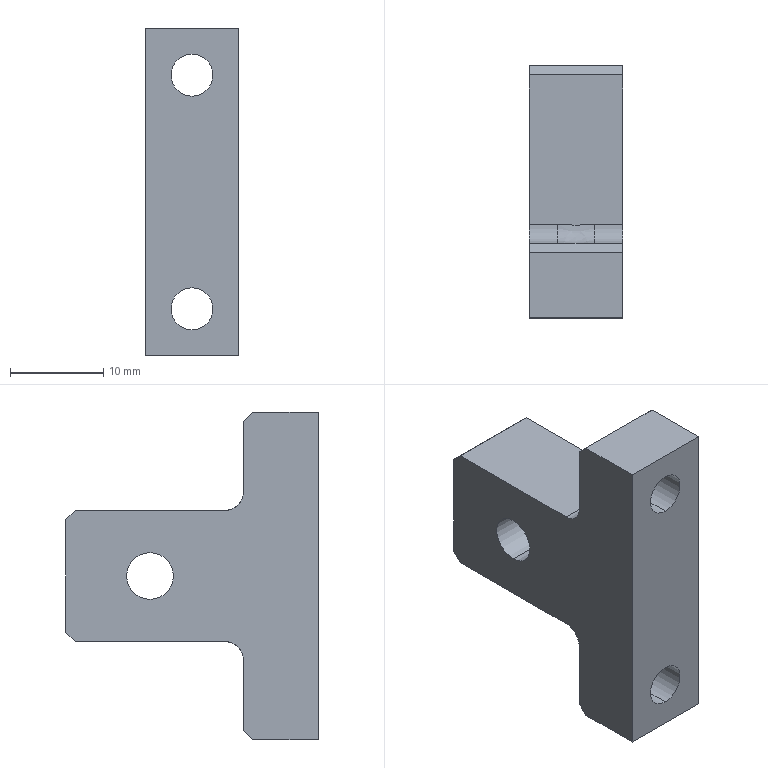Part | SolidWorks | features HoleWzd 2, Chamfer 1, Extrusion 1, Fillet 1 | 1 solid | 34 faces | box 10 x 27 x 35 mm | volume 4690 mm3 | plane 18 | cylinder 14 | spline 2 | commonest cylinder face diameters 4 x4 4.5 x4 8 x4 5 x2
STEP:
#1=CARTESIAN_POINT('',(-5.,18.,2.5));
#2=VERTEX_POINT('',#1);
#3=CARTESIAN_POINT('',(-5.,18.,-2.5));
#4=VERTEX_POINT('',#3);
#5=CARTESIAN_POINT('',(-5.,18.,0.));
#6=DIRECTION('',(1.,0.,0.));
#7=DIRECTION('',(0.,0.,-1.));
#8=AXIS2_PLACEMENT_3D('',#5,#6,#7);
#9=CIRCLE('',#8,2.5);
#10=EDGE_CURVE('',#2,#4,#9,.T.);
#11=ORIENTED_EDGE('',*,*,#10,.F.);
#12=CARTESIAN_POINT('',(5.,18.,2.5));
#13=VERTEX_POINT('',#12);
#14=CARTESIAN_POINT('',(5.,18.,2.5));
#15=DIRECTION('',(1.,0.,0.));
#16=VECTOR('',#15,1000.);
#17=LINE('',#14,#16);
#18=EDGE_CURVE('',#2,#13,#17,.T.);
#19=ORIENTED_EDGE('',*,*,#18,.T.);
#20=CARTESIAN_POINT('',(5.,18.,-2.5));
#21=VERTEX_POINT('',#20);
#22=CARTESIAN_POINT('',(5.,18.,0.));
#23=DIRECTION('',(1.,0.,0.));
#24=DIRECTION('',(0.,0.,-1.));
#25=AXIS2_PLACEMENT_3D('',#22,#23,#24);
#26=CIRCLE('',#25,2.5);
#27=EDGE_CURVE('',#13,#21,#26,.T.);
#28=ORIENTED_EDGE('',*,*,#27,.T.);
#29=CARTESIAN_POINT('',(5.,18.,-2.5));
#30=DIRECTION('',(1.,0.,0.));
#31=VECTOR('',#30,1000.);
#32=LINE('',#29,#31);
#33=EDGE_CURVE('',#4,#21,#32,.T.);
#34=ORIENTED_EDGE('',*,*,#33,.F.);
#35=EDGE_LOOP('',(#11,#19,#28,#34));
#36=FACE_OUTER_BOUND('',#35,.T.);
#37=CARTESIAN_POINT('',(5.,18.,0.));
#38=DIRECTION('',(1.,0.,0.));
#39=DIRECTION('',(0.,0.,-1.));
#40=AXIS2_PLACEMENT_3D('',#37,#38,#39);
#41=CYLINDRICAL_SURFACE('',#40,2.5);
#42=ADVANCED_FACE('',(#36),#41,.F.);
#43=CARTESIAN_POINT('',(0.,3.4,-16.5));
#44=VERTEX_POINT('',#43);
#45=CARTESIAN_POINT('',(0.,3.4,-8.5));
#46=VERTEX_POINT('',#45);
#47=CARTESIAN_POINT('',(0.,3.4,-12.5));
#48=DIRECTION('',(0.,1.,0.));
#49=DIRECTION('',(0.,0.,1.));
#50=AXIS2_PLACEMENT_3D('',#47,#48,#49);
#51=CIRCLE('',#50,4.);
#52=EDGE_CURVE('',#44,#46,#51,.T.);
#53=ORIENTED_EDGE('',*,*,#52,.F.);
#54=CARTESIAN_POINT('',(0.,8.,-16.5));
#55=VERTEX_POINT('',#54);
#56=CARTESIAN_POINT('',(0.,8.,-16.5));
#57=DIRECTION('',(0.,1.,0.));
#58=VECTOR('',#57,1000.);
#59=LINE('',#56,#58);
#60=EDGE_CURVE('',#44,#55,#59,.T.);
#61=ORIENTED_EDGE('',*,*,#60,.T.);
#62=CARTESIAN_POINT('',(-1.936,8.,-9.));
#63=VERTEX_POINT('',#62);
#64=CARTESIAN_POINT('',(0.,8.,-12.5));
#65=DIRECTION('',(0.,1.,0.));
#66=DIRECTION('',(0.,0.,1.));
#67=AXIS2_PLACEMENT_3D('',#64,#65,#66);
#68=CIRCLE('',#67,4.);
#69=EDGE_CURVE('',#55,#63,#68,.T.);
#70=ORIENTED_EDGE('',*,*,#69,.T.);
#71=CARTESIAN_POINT('',(0.,8.,-8.5));
#72=VERTEX_POINT('',#71);
#73=CARTESIAN_POINT('',(0.,8.,-12.5));
#74=DIRECTION('',(0.,1.,0.));
#75=DIRECTION('',(0.,0.,1.));
#76=AXIS2_PLACEMENT_3D('',#73,#74,#75);
#77=CIRCLE('',#76,4.);
#78=EDGE_CURVE('',#63,#72,#77,.T.);
#79=ORIENTED_EDGE('',*,*,#78,.T.);
#80=CARTESIAN_POINT('',(0.,8.,-8.5));
#81=DIRECTION('',(0.,1.,0.));
#82=VECTOR('',#81,1000.);
#83=LINE('',#80,#82);
#84=EDGE_CURVE('',#46,#72,#83,.T.);
#85=ORIENTED_EDGE('',*,*,#84,.F.);
#86=EDGE_LOOP('',(#53,#61,#70,#79,#85));
#87=FACE_OUTER_BOUND('',#86,.T.);
#88=CARTESIAN_POINT('',(0.,8.,-12.5));
#89=DIRECTION('',(0.,1.,0.));
#90=DIRECTION('',(0.,0.,1.));
#91=AXIS2_PLACEMENT_3D('',#88,#89,#90);
#92=CYLINDRICAL_SURFACE('',#91,4.);
#93=ADVANCED_FACE('',(#87),#92,.F.);
#94=CARTESIAN_POINT('',(0.,0.,-14.75));
#95=VERTEX_POINT('',#94);
#96=CARTESIAN_POINT('',(0.,0.,-10.25));
#97=VERTEX_POINT('',#96);
#98=CARTESIAN_POINT('',(0.,0.,-12.5));
#99=DIRECTION('',(0.,1.,0.));
#100=DIRECTION('',(0.,0.,1.));
#101=AXIS2_PLACEMENT_3D('',#98,#99,#100);
#102=CIRCLE('',#101,2.25);
#103=EDGE_CURVE('',#95,#97,#102,.T.);
#104=ORIENTED_EDGE('',*,*,#103,.F.);
#105=CARTESIAN_POINT('',(0.,3.4,-14.75));
#106=VERTEX_POINT('',#105);
#107=CARTESIAN_POINT('',(0.,8.,-14.75));
#108=DIRECTION('',(0.,1.,0.));
#109=VECTOR('',#108,1000.);
#110=LINE('',#107,#109);
#111=EDGE_CURVE('',#95,#106,#110,.T.);
#112=ORIENTED_EDGE('',*,*,#111,.T.);
#113=CARTESIAN_POINT('',(0.,3.4,-10.25));
#114=VERTEX_POINT('',#113);
#115=CARTESIAN_POINT('',(0.,3.4,-12.5));
#116=DIRECTION('',(0.,1.,0.));
#117=DIRECTION('',(0.,0.,1.));
#118=AXIS2_PLACEMENT_3D('',#115,#116,#117);
#119=CIRCLE('',#118,2.25);
#120=EDGE_CURVE('',#106,#114,#119,.T.);
#121=ORIENTED_EDGE('',*,*,#120,.T.);
#122=CARTESIAN_POINT('',(0.,8.,-10.25));
#123=DIRECTION('',(0.,1.,0.));
#124=VECTOR('',#123,1000.);
#125=LINE('',#122,#124);
#126=EDGE_CURVE('',#97,#114,#125,.T.);
#127=ORIENTED_EDGE('',*,*,#126,.F.);
#128=EDGE_LOOP('',(#104,#112,#121,#127));
#129=FACE_OUTER_BOUND('',#128,.T.);
#130=CARTESIAN_POINT('',(0.,8.,-12.5));
#131=DIRECTION('',(0.,1.,0.));
#132=DIRECTION('',(0.,0.,1.));
#133=AXIS2_PLACEMENT_3D('',#130,#131,#132);
#134=CYLINDRICAL_SURFACE('',#133,2.25);
#135=ADVANCED_FACE('',(#129),#134,.F.);
#136=CARTESIAN_POINT('',(0.,3.4,8.5));
#137=VERTEX_POINT('',#136);
#138=CARTESIAN_POINT('',(0.,3.4,16.5));
#139=VERTEX_POINT('',#138);
#140=CARTESIAN_POINT('',(0.,3.4,12.5));
#141=DIRECTION('',(0.,1.,0.));
#142=DIRECTION('',(0.,0.,1.));
#143=AXIS2_PLACEMENT_3D('',#140,#141,#142);
#144=CIRCLE('',#143,4.);
#145=EDGE_CURVE('',#137,#139,#144,.T.);
#146=ORIENTED_EDGE('',*,*,#145,.F.);
#147=CARTESIAN_POINT('',(0.,8.,8.5));
#148=VERTEX_POINT('',#147);
#149=CARTESIAN_POINT('',(0.,8.,8.5));
#150=DIRECTION('',(0.,1.,0.));
#151=VECTOR('',#150,1000.);
#152=LINE('',#149,#151);
#153=EDGE_CURVE('',#137,#148,#152,.T.);
#154=ORIENTED_EDGE('',*,*,#153,.T.);
#155=CARTESIAN_POINT('',(-1.936,8.,9.));
#156=VERTEX_POINT('',#155);
#157=CARTESIAN_POINT('',(0.,8.,12.5));
#158=DIRECTION('',(0.,1.,0.));
#159=DIRECTION('',(0.,0.,1.));
#160=AXIS2_PLACEMENT_3D('',#157,#158,#159);
#161=CIRCLE('',#160,4.);
#162=EDGE_CURVE('',#148,#156,#161,.T.);
#163=ORIENTED_EDGE('',*,*,#162,.T.);
#164=CARTESIAN_POINT('',(0.,8.,16.5));
#165=VERTEX_POINT('',#164);
#166=CARTESIAN_POINT('',(0.,8.,12.5));
#167=DIRECTION('',(0.,1.,0.));
#168=DIRECTION('',(0.,0.,1.));
#169=AXIS2_PLACEMENT_3D('',#166,#167,#168);
#170=CIRCLE('',#169,4.);
#171=EDGE_CURVE('',#156,#165,#170,.T.);
#172=ORIENTED_EDGE('',*,*,#171,.T.);
#173=CARTESIAN_POINT('',(0.,8.,16.5));
#174=DIRECTION('',(0.,1.,0.));
#175=VECTOR('',#174,1000.);
#176=LINE('',#173,#175);
#177=EDGE_CURVE('',#139,#165,#176,.T.);
#178=ORIENTED_EDGE('',*,*,#177,.F.);
#179=EDGE_LOOP('',(#146,#154,#163,#172,#178));
#180=FACE_OUTER_BOUND('',#179,.T.);
#181=CARTESIAN_POINT('',(0.,8.,12.5));
#182=DIRECTION('',(0.,1.,0.));
#183=DIRECTION('',(0.,0.,1.));
#184=AXIS2_PLACEMENT_3D('',#181,#182,#183);
#185=CYLINDRICAL_SURFACE('',#184,4.);
#186=ADVANCED_FACE('',(#180),#185,.F.);
#187=CARTESIAN_POINT('',(0.,0.,10.25));
#188=VERTEX_POINT('',#187);
#189=CARTESIAN_POINT('',(0.,0.,14.75));
#190=VERTEX_POINT('',#189);
#191=CARTESIAN_POINT('',(0.,0.,12.5));
#192=DIRECTION('',(0.,1.,0.));
#193=DIRECTION('',(0.,0.,1.));
#194=AXIS2_PLACEMENT_3D('',#191,#192,#193);
#195=CIRCLE('',#194,2.25);
#196=EDGE_CURVE('',#188,#190,#195,.T.);
#197=ORIENTED_EDGE('',*,*,#196,.F.);
#198=CARTESIAN_POINT('',(0.,3.4,10.25));
#199=VERTEX_POINT('',#198);
#200=CARTESIAN_POINT('',(0.,8.,10.25));
#201=DIRECTION('',(0.,1.,0.));
#202=VECTOR('',#201,1000.);
#203=LINE('',#200,#202);
#204=EDGE_CURVE('',#188,#199,#203,.T.);
#205=ORIENTED_EDGE('',*,*,#204,.T.);
#206=CARTESIAN_POINT('',(0.,3.4,14.75));
#207=VERTEX_POINT('',#206);
#208=CARTESIAN_POINT('',(0.,3.4,12.5));
#209=DIRECTION('',(0.,1.,0.));
#210=DIRECTION('',(0.,0.,1.));
#211=AXIS2_PLACEMENT_3D('',#208,#209,#210);
#212=CIRCLE('',#211,2.25);
#213=EDGE_CURVE('',#199,#207,#212,.T.);
#214=ORIENTED_EDGE('',*,*,#213,.T.);
#215=CARTESIAN_POINT('',(0.,8.,14.75));
#216=DIRECTION('',(0.,1.,0.));
#217=VECTOR('',#216,1000.);
#218=LINE('',#215,#217);
#219=EDGE_CURVE('',#190,#207,#218,.T.);
#220=ORIENTED_EDGE('',*,*,#219,.F.);
#221=EDGE_LOOP('',(#197,#205,#214,#220));
#222=FACE_OUTER_BOUND('',#221,.T.);
#223=CARTESIAN_POINT('',(0.,8.,12.5));
#224=DIRECTION('',(0.,1.,0.));
#225=DIRECTION('',(0.,0.,1.));
#226=AXIS2_PLACEMENT_3D('',#223,#224,#225);
#227=CYLINDRICAL_SURFACE('',#226,2.25);
#228=ADVANCED_FACE('',(#222),#227,.F.);
#229=CARTESIAN_POINT('',(5.,8.,9.));
#230=VERTEX_POINT('',#229);
#231=CARTESIAN_POINT('',(5.,8.,16.5));
#232=VERTEX_POINT('',#231);
#233=CARTESIAN_POINT('',(5.,8.,7.));
#234=DIRECTION('',(0.,0.,1.));
#235=VECTOR('',#234,1000.);
#236=LINE('',#233,#235);
#237=EDGE_CURVE('',#230,#232,#236,.T.);
#238=ORIENTED_EDGE('',*,*,#237,.F.);
#239=CARTESIAN_POINT('',(1.936,8.,9.));
#240=VERTEX_POINT('',#239);
#241=CARTESIAN_POINT('',(-5.,8.,9.));
#242=DIRECTION('',(-1.,0.,0.));
#243=VECTOR('',#242,1000.);
#244=LINE('',#241,#243);
#245=EDGE_CURVE('',#230,#240,#244,.T.);
#246=ORIENTED_EDGE('',*,*,#245,.T.);
#247=CARTESIAN_POINT('',(0.,8.,12.5));
#248=DIRECTION('',(0.,1.,0.));
#249=DIRECTION('',(0.,0.,1.));
#250=AXIS2_PLACEMENT_3D('',#247,#248,#249);
#251=CIRCLE('',#250,4.);
#252=EDGE_CURVE('',#165,#240,#251,.T.);
#253=ORIENTED_EDGE('',*,*,#252,.F.);
#254=CARTESIAN_POINT('',(5.,8.,16.5));
#255=DIRECTION('',(1.,0.,0.));
#256=VECTOR('',#255,1000.);
#257=LINE('',#254,#256);
#258=EDGE_CURVE('',#165,#232,#257,.T.);
#259=ORIENTED_EDGE('',*,*,#258,.T.);
#260=EDGE_LOOP('',(#238,#246,#253,#259));
#261=FACE_OUTER_BOUND('',#260,.T.);
#262=CARTESIAN_POINT('',(5.,8.,7.));
#263=DIRECTION('',(0.,-1.,0.));
#264=DIRECTION('',(0.,0.,-1.));
#265=AXIS2_PLACEMENT_3D('',#262,#263,#264);
#266=PLANE('',#265);
#267=ADVANCED_FACE('',(#261),#266,.F.);
#268=CARTESIAN_POINT('',(-5.,8.,-16.5));
#269=VERTEX_POINT('',#268);
#270=CARTESIAN_POINT('',(-5.,8.,-9.));
#271=VERTEX_POINT('',#270);
#272=CARTESIAN_POINT('',(-5.,8.,-17.5));
#273=DIRECTION('',(0.,0.,1.));
#274=VECTOR('',#273,1000.);
#275=LINE('',#272,#274);
#276=EDGE_CURVE('',#269,#271,#275,.T.);
#277=ORIENTED_EDGE('',*,*,#276,.T.);
#278=CARTESIAN_POINT('',(5.,8.,-9.));
#279=DIRECTION('',(1.,0.,0.));
#280=VECTOR('',#279,1000.);
#281=LINE('',#278,#280);
#282=EDGE_CURVE('',#271,#63,#281,.T.);
#283=ORIENTED_EDGE('',*,*,#282,.T.);
#284=ORIENTED_EDGE('',*,*,#69,.F.);
#285=CARTESIAN_POINT('',(5.,8.,-16.5));
#286=DIRECTION('',(-1.,0.,0.));
#287=VECTOR('',#286,1000.);
#288=LINE('',#285,#287);
#289=EDGE_CURVE('',#55,#269,#288,.T.);
#290=ORIENTED_EDGE('',*,*,#289,.T.);
#291=EDGE_LOOP('',(#277,#283,#284,#290));
#292=FACE_OUTER_BOUND('',#291,.T.);
#293=CARTESIAN_POINT('',(5.,8.,-17.5));
#294=DIRECTION('',(0.,-1.,0.));
#295=DIRECTION('',(0.,0.,-1.));
#296=AXIS2_PLACEMENT_3D('',#293,#294,#295);
#297=PLANE('',#296);
#298=ADVANCED_FACE('',(#292),#297,.F.);
#299=CARTESIAN_POINT('',(5.,7.,17.5));
#300=VERTEX_POINT('',#299);
#301=CARTESIAN_POINT('',(5.,0.,17.5));
#302=VERTEX_POINT('',#301);
#303=CARTESIAN_POINT('',(5.,8.,17.5));
#304=DIRECTION('',(0.,-1.,0.));
#305=VECTOR('',#304,1000.);
#306=LINE('',#303,#305);
#307=EDGE_CURVE('',#300,#302,#306,.T.);
#308=ORIENTED_EDGE('',*,*,#307,.F.);
#309=CARTESIAN_POINT('',(-5.,7.,17.5));
#310=VERTEX_POINT('',#309);
#311=CARTESIAN_POINT('',(5.,7.,17.5));
#312=DIRECTION('',(-1.,0.,0.));
#313=VECTOR('',#312,1000.);
#314=LINE('',#311,#313);
#315=EDGE_CURVE('',#300,#310,#314,.T.);
#316=ORIENTED_EDGE('',*,*,#315,.T.);
#317=CARTESIAN_POINT('',(-5.,0.,17.5));
#318=VERTEX_POINT('',#317);
#319=CARTESIAN_POINT('',(-5.,8.,17.5));
#320=DIRECTION('',(0.,-1.,0.));
#321=VECTOR('',#320,1000.);
#322=LINE('',#319,#321);
#323=EDGE_CURVE('',#310,#318,#322,.T.);
#324=ORIENTED_EDGE('',*,*,#323,.T.);
#325=CARTESIAN_POINT('',(5.,0.,17.5));
#326=DIRECTION('',(-1.,0.,0.));
#327=VECTOR('',#326,1000.);
#328=LINE('',#325,#327);
#329=EDGE_CURVE('',#302,#318,#328,.T.);
#330=ORIENTED_EDGE('',*,*,#329,.F.);
#331=EDGE_LOOP('',(#308,#316,#324,#330));
#332=FACE_OUTER_BOUND('',#331,.T.);
#333=CARTESIAN_POINT('',(5.,8.,17.5));
#334=DIRECTION('',(0.,0.,-1.));
#335=DIRECTION('',(-1.,0.,0.));
#336=AXIS2_PLACEMENT_3D('',#333,#334,#335);
#337=PLANE('',#336);
#338=ADVANCED_FACE('',(#332),#337,.F.);
#339=CARTESIAN_POINT('',(0.,0.,-12.5));
#340=DIRECTION('',(0.,1.,0.));
#341=DIRECTION('',(0.,0.,1.));
#342=AXIS2_PLACEMENT_3D('',#339,#340,#341);
#343=CIRCLE('',#342,2.25);
#344=EDGE_CURVE('',#97,#95,#343,.T.);
#345=ORIENTED_EDGE('',*,*,#344,.T.);
#346=ORIENTED_EDGE('',*,*,#103,.T.);
#347=EDGE_LOOP('',(#345,#346));
#348=FACE_BOUND('',#347,.T.);
#349=CARTESIAN_POINT('',(0.,0.,12.5));
#350=DIRECTION('',(0.,1.,0.));
#351=DIRECTION('',(0.,0.,1.));
#352=AXIS2_PLACEMENT_3D('',#349,#350,#351);
#353=CIRCLE('',#352,2.25);
#354=EDGE_CURVE('',#190,#188,#353,.T.);
#355=ORIENTED_EDGE('',*,*,#354,.T.);
#356=ORIENTED_EDGE('',*,*,#196,.T.);
#357=EDGE_LOOP('',(#355,#356));
#358=FACE_BOUND('',#357,.T.);
#359=CARTESIAN_POINT('',(-5.,0.,-17.5));
#360=VERTEX_POINT('',#359);
#361=CARTESIAN_POINT('',(-5.,0.,17.5));
#362=DIRECTION('',(0.,0.,-1.));
#363=VECTOR('',#362,1000.);
#364=LINE('',#361,#363);
#365=EDGE_CURVE('',#318,#360,#364,.T.);
#366=ORIENTED_EDGE('',*,*,#365,.T.);
#367=CARTESIAN_POINT('',(5.,0.,-17.5));
#368=VERTEX_POINT('',#367);
#369=CARTESIAN_POINT('',(5.,0.,-17.5));
#370=DIRECTION('',(-1.,0.,0.));
#371=VECTOR('',#370,1000.);
#372=LINE('',#369,#371);
#373=EDGE_CURVE('',#368,#360,#372,.T.);
#374=ORIENTED_EDGE('',*,*,#373,.F.);
#375=CARTESIAN_POINT('',(5.,0.,17.5));
#376=DIRECTION('',(0.,0.,-1.));
#377=VECTOR('',#376,1000.);
#378=LINE('',#375,#377);
#379=EDGE_CURVE('',#302,#368,#378,.T.);
#380=ORIENTED_EDGE('',*,*,#379,.F.);
#381=ORIENTED_EDGE('',*,*,#329,.T.);
#382=EDGE_LOOP('',(#366,#374,#380,#381));
#383=FACE_OUTER_BOUND('',#382,.T.);
#384=CARTESIAN_POINT('',(5.,0.,17.5));
#385=DIRECTION('',(0.,1.,0.));
#386=DIRECTION('',(0.,0.,1.));
#387=AXIS2_PLACEMENT_3D('',#384,#385,#386);
#388=PLANE('',#387);
#389=ADVANCED_FACE('',(#348,#358,#383),#388,.F.);
#390=CARTESIAN_POINT('',(-5.,7.,-17.5));
#391=VERTEX_POINT('',#390);
#392=CARTESIAN_POINT('',(-5.,0.,-17.5));
#393=DIRECTION('',(0.,1.,0.));
#394=VECTOR('',#393,1000.);
#395=LINE('',#392,#394);
#396=EDGE_CURVE('',#360,#391,#395,.T.);
#397=ORIENTED_EDGE('',*,*,#396,.T.);
#398=CARTESIAN_POINT('',(5.,7.,-17.5));
#399=VERTEX_POINT('',#398);
#400=CARTESIAN_POINT('',(5.,7.,-17.5));
#401=DIRECTION('',(1.,0.,0.));
#402=VECTOR('',#401,1000.);
#403=LINE('',#400,#402);
#404=EDGE_CURVE('',#391,#399,#403,.T.);
#405=ORIENTED_EDGE('',*,*,#404,.T.);
#406=CARTESIAN_POINT('',(5.,0.,-17.5));
#407=DIRECTION('',(0.,1.,0.));
#408=VECTOR('',#407,1000.);
#409=LINE('',#406,#408);
#410=EDGE_CURVE('',#368,#399,#409,.T.);
#411=ORIENTED_EDGE('',*,*,#410,.F.);
#412=ORIENTED_EDGE('',*,*,#373,.T.);
#413=EDGE_LOOP('',(#397,#405,#411,#412));
#414=FACE_OUTER_BOUND('',#413,.T.);
#415=CARTESIAN_POINT('',(5.,0.,-17.5));
#416=DIRECTION('',(0.,0.,1.));
#417=DIRECTION('',(1.,0.,0.));
#418=AXIS2_PLACEMENT_3D('',#415,#416,#417);
#419=PLANE('',#418);
#420=ADVANCED_FACE('',(#414),#419,.F.);
#421=CARTESIAN_POINT('',(1.936,8.,-9.));
#422=VERTEX_POINT('',#421);
#423=CARTESIAN_POINT('',(0.,8.,-12.5));
#424=DIRECTION('',(0.,1.,0.));
#425=DIRECTION('',(0.,0.,1.));
#426=AXIS2_PLACEMENT_3D('',#423,#424,#425);
#427=CIRCLE('',#426,4.);
#428=EDGE_CURVE('',#422,#55,#427,.T.);
#429=ORIENTED_EDGE('',*,*,#428,.F.);
#430=CARTESIAN_POINT('',(5.,8.,-9.));
#431=VERTEX_POINT('',#430);
#432=CARTESIAN_POINT('',(5.,8.,-9.));
#433=DIRECTION('',(1.,0.,0.));
#434=VECTOR('',#433,1000.);
#435=LINE('',#432,#434);
#436=EDGE_CURVE('',#422,#431,#435,.T.);
#437=ORIENTED_EDGE('',*,*,#436,.T.);
#438=CARTESIAN_POINT('',(5.,8.,-16.5));
#439=VERTEX_POINT('',#438);
#440=CARTESIAN_POINT('',(5.,8.,-17.5));
#441=DIRECTION('',(0.,0.,1.));
#442=VECTOR('',#441,1000.);
#443=LINE('',#440,#442);
#444=EDGE_CURVE('',#439,#431,#443,.T.);
#445=ORIENTED_EDGE('',*,*,#444,.F.);
#446=CARTESIAN_POINT('',(5.,8.,-16.5));
#447=DIRECTION('',(-1.,0.,0.));
#448=VECTOR('',#447,1000.);
#449=LINE('',#446,#448);
#450=EDGE_CURVE('',#439,#55,#449,.T.);
#451=ORIENTED_EDGE('',*,*,#450,.T.);
#452=EDGE_LOOP('',(#429,#437,#445,#451));
#453=FACE_OUTER_BOUND('',#452,.T.);
#454=CARTESIAN_POINT('',(5.,8.,-17.5));
#455=DIRECTION('',(0.,-1.,0.));
#456=DIRECTION('',(0.,0.,-1.));
#457=AXIS2_PLACEMENT_3D('',#454,#455,#456);
#458=PLANE('',#457);
#459=ADVANCED_FACE('',(#453),#458,.F.);
#460=CARTESIAN_POINT('',(5.,10.,-7.));
#461=VERTEX_POINT('',#460);
#462=CARTESIAN_POINT('',(5.,26.,-7.));
#463=VERTEX_POINT('',#462);
#464=CARTESIAN_POINT('',(5.,8.,-7.));
#465=DIRECTION('',(0.,1.,0.));
#466=VECTOR('',#465,1000.);
#467=LINE('',#464,#466);
#468=EDGE_CURVE('',#461,#463,#467,.T.);
#469=ORIENTED_EDGE('',*,*,#468,.F.);
#470=CARTESIAN_POINT('',(1.936,10.,-7.));
#471=VERTEX_POINT('',#470);
#472=CARTESIAN_POINT('',(-5.,10.,-7.));
#473=DIRECTION('',(-1.,0.,0.));
#474=VECTOR('',#473,1000.);
#475=LINE('',#472,#474);
#476=EDGE_CURVE('',#461,#471,#475,.T.);
#477=ORIENTED_EDGE('',*,*,#476,.T.);
#478=CARTESIAN_POINT('',(-1.936,10.,-7.));
#479=VERTEX_POINT('',#478);
#480=CARTESIAN_POINT('',(1.936,10.,-7.));
#481=CARTESIAN_POINT('',(1.614,10.,-7.));
#482=CARTESIAN_POINT('',(1.291,9.982,-7.));
#483=CARTESIAN_POINT('',(0.6464,9.95,-7.));
#484=CARTESIAN_POINT('',(0.3239,9.937,-7.));
#485=CARTESIAN_POINT('',(-0.3219,9.936,-7.));
#486=CARTESIAN_POINT('',(-0.645,9.95,-7.));
#487=CARTESIAN_POINT('',(-1.29,9.982,-7.));
#488=CARTESIAN_POINT('',(-1.613,10.,-7.));
#489=CARTESIAN_POINT('',(-1.936,10.,-7.));
#490=B_SPLINE_CURVE_WITH_KNOTS('',3,(#480,#481,#482,#483,#484,#485,#486,#487,#488,#489),.UNSPECIFIED.,.F.,.F.,(4,2,2,2,4),(0.,0.0009685,0.001937,0.002906,0.003874),.UNSPECIFIED.);
#491=EDGE_CURVE('',#471,#479,#490,.T.);
#492=ORIENTED_EDGE('',*,*,#491,.T.);
#493=CARTESIAN_POINT('',(-5.,10.,-7.));
#494=VERTEX_POINT('',#493);
#495=CARTESIAN_POINT('',(-5.,10.,-7.));
#496=DIRECTION('',(-1.,0.,0.));
#497=VECTOR('',#496,1000.);
#498=LINE('',#495,#497);
#499=EDGE_CURVE('',#479,#494,#498,.T.);
#500=ORIENTED_EDGE('',*,*,#499,.T.);
#501=CARTESIAN_POINT('',(-5.,26.,-7.));
#502=VERTEX_POINT('',#501);
#503=CARTESIAN_POINT('',(-5.,8.,-7.));
#504=DIRECTION('',(0.,1.,0.));
#505=VECTOR('',#504,1000.);
#506=LINE('',#503,#505);
#507=EDGE_CURVE('',#494,#502,#506,.T.);
#508=ORIENTED_EDGE('',*,*,#507,.T.);
#509=CARTESIAN_POINT('',(5.,26.,-7.));
#510=DIRECTION('',(1.,0.,0.));
#511=VECTOR('',#510,1000.);
#512=LINE('',#509,#511);
#513=EDGE_CURVE('',#502,#463,#512,.T.);
#514=ORIENTED_EDGE('',*,*,#513,.T.);
#515=EDGE_LOOP('',(#469,#477,#492,#500,#508,#514));
#516=FACE_OUTER_BOUND('',#515,.T.);
#517=CARTESIAN_POINT('',(5.,8.,-7.));
#518=DIRECTION('',(0.,0.,1.));
#519=DIRECTION('',(0.,-1.,0.));
#520=AXIS2_PLACEMENT_3D('',#517,#518,#519);
#521=PLANE('',#520);
#522=ADVANCED_FACE('',(#516),#521,.F.);
#523=CARTESIAN_POINT('',(-5.,27.,-6.));
#524=VERTEX_POINT('',#523);
#525=CARTESIAN_POINT('',(-5.,27.,6.));
#526=VERTEX_POINT('',#525);
#527=CARTESIAN_POINT('',(-5.,27.,-7.));
#528=DIRECTION('',(0.,0.,1.));
#529=VECTOR('',#528,1000.);
#530=LINE('',#527,#529);
#531=EDGE_CURVE('',#524,#526,#530,.T.);
#532=ORIENTED_EDGE('',*,*,#531,.T.);
#533=CARTESIAN_POINT('',(5.,27.,6.));
#534=VERTEX_POINT('',#533);
#535=CARTESIAN_POINT('',(5.,27.,6.));
#536=DIRECTION('',(1.,0.,0.));
#537=VECTOR('',#536,1000.);
#538=LINE('',#535,#537);
#539=EDGE_CURVE('',#526,#534,#538,.T.);
#540=ORIENTED_EDGE('',*,*,#539,.T.);
#541=CARTESIAN_POINT('',(5.,27.,-6.));
#542=VERTEX_POINT('',#541);
#543=CARTESIAN_POINT('',(5.,27.,-7.));
#544=DIRECTION('',(0.,0.,1.));
#545=VECTOR('',#544,1000.);
#546=LINE('',#543,#545);
#547=EDGE_CURVE('',#542,#534,#546,.T.);
#548=ORIENTED_EDGE('',*,*,#547,.F.);
#549=CARTESIAN_POINT('',(5.,27.,-6.));
#550=DIRECTION('',(-1.,0.,0.));
#551=VECTOR('',#550,1000.);
#552=LINE('',#549,#551);
#553=EDGE_CURVE('',#542,#524,#552,.T.);
#554=ORIENTED_EDGE('',*,*,#553,.T.);
#555=EDGE_LOOP('',(#532,#540,#548,#554));
#556=FACE_OUTER_BOUND('',#555,.T.);
#557=CARTESIAN_POINT('',(5.,27.,-7.));
#558=DIRECTION('',(0.,-1.,0.));
#559=DIRECTION('',(0.,0.,-1.));
#560=AXIS2_PLACEMENT_3D('',#557,#558,#559);
#561=PLANE('',#560);
#562=ADVANCED_FACE('',(#556),#561,.F.);
#563=CARTESIAN_POINT('',(-5.,26.,7.));
#564=VERTEX_POINT('',#563);
#565=CARTESIAN_POINT('',(-5.,10.,7.));
#566=VERTEX_POINT('',#565);
#567=CARTESIAN_POINT('',(-5.,27.,7.));
#568=DIRECTION('',(0.,-1.,0.));
#569=VECTOR('',#568,1000.);
#570=LINE('',#567,#569);
#571=EDGE_CURVE('',#564,#566,#570,.T.);
#572=ORIENTED_EDGE('',*,*,#571,.T.);
#573=CARTESIAN_POINT('',(-1.936,10.,7.));
#574=VERTEX_POINT('',#573);
#575=CARTESIAN_POINT('',(5.,10.,7.));
#576=DIRECTION('',(1.,0.,0.));
#577=VECTOR('',#576,1000.);
#578=LINE('',#575,#577);
#579=EDGE_CURVE('',#566,#574,#578,.T.);
#580=ORIENTED_EDGE('',*,*,#579,.T.);
#581=CARTESIAN_POINT('',(1.936,10.,7.));
#582=VERTEX_POINT('',#581);
#583=CARTESIAN_POINT('',(-1.936,10.,7.));
#584=CARTESIAN_POINT('',(-1.613,10.,7.));
#585=CARTESIAN_POINT('',(-1.29,9.982,7.));
#586=CARTESIAN_POINT('',(-0.645,9.95,7.));
#587=CARTESIAN_POINT('',(-0.3219,9.936,7.));
#588=CARTESIAN_POINT('',(0.3238,9.937,7.));
#589=CARTESIAN_POINT('',(0.6463,9.95,7.));
#590=CARTESIAN_POINT('',(1.291,9.982,7.));
#591=CARTESIAN_POINT('',(1.614,10.,7.));
#592=CARTESIAN_POINT('',(1.936,10.,7.));
#593=B_SPLINE_CURVE_WITH_KNOTS('',3,(#583,#584,#585,#586,#587,#588,#589,#590,#591,#592),.UNSPECIFIED.,.F.,.F.,(4,2,2,2,4),(0.,0.0009697,0.001939,0.002909,0.003879),.UNSPECIFIED.);
#594=EDGE_CURVE('',#574,#582,#593,.T.);
#595=ORIENTED_EDGE('',*,*,#594,.T.);
#596=CARTESIAN_POINT('',(5.,10.,7.));
#597=VERTEX_POINT('',#596);
#598=CARTESIAN_POINT('',(5.,10.,7.));
#599=DIRECTION('',(1.,0.,0.));
#600=VECTOR('',#599,1000.);
#601=LINE('',#598,#600);
#602=EDGE_CURVE('',#582,#597,#601,.T.);
#603=ORIENTED_EDGE('',*,*,#602,.T.);
#604=CARTESIAN_POINT('',(5.,26.,7.));
#605=VERTEX_POINT('',#604);
#606=CARTESIAN_POINT('',(5.,27.,7.));
#607=DIRECTION('',(0.,-1.,0.));
#608=VECTOR('',#607,1000.);
#609=LINE('',#606,#608);
#610=EDGE_CURVE('',#605,#597,#609,.T.);
#611=ORIENTED_EDGE('',*,*,#610,.F.);
#612=CARTESIAN_POINT('',(5.,26.,7.));
#613=DIRECTION('',(-1.,0.,0.));
#614=VECTOR('',#613,1000.);
#615=LINE('',#612,#614);
#616=EDGE_CURVE('',#605,#564,#615,.T.);
#617=ORIENTED_EDGE('',*,*,#616,.T.);
#618=EDGE_LOOP('',(#572,#580,#595,#603,#611,#617));
#619=FACE_OUTER_BOUND('',#618,.T.);
#620=CARTESIAN_POINT('',(5.,27.,7.));
#621=DIRECTION('',(0.,0.,-1.));
#622=DIRECTION('',(0.,1.,0.));
#623=AXIS2_PLACEMENT_3D('',#620,#621,#622);
#624=PLANE('',#623);
#625=ADVANCED_FACE('',(#619),#624,.F.);
#626=ORIENTED_EDGE('',*,*,#171,.F.);
#627=CARTESIAN_POINT('',(-5.,8.,9.));
#628=VERTEX_POINT('',#627);
#629=CARTESIAN_POINT('',(-5.,8.,9.));
#630=DIRECTION('',(-1.,0.,0.));
#631=VECTOR('',#630,1000.);
#632=LINE('',#629,#631);
#633=EDGE_CURVE('',#156,#628,#632,.T.);
#634=ORIENTED_EDGE('',*,*,#633,.T.);
#635=CARTESIAN_POINT('',(-5.,8.,16.5));
#636=VERTEX_POINT('',#635);
#637=CARTESIAN_POINT('',(-5.,8.,7.));
#638=DIRECTION('',(0.,0.,1.));
#639=VECTOR('',#638,1000.);
#640=LINE('',#637,#639);
#641=EDGE_CURVE('',#628,#636,#640,.T.);
#642=ORIENTED_EDGE('',*,*,#641,.T.);
#643=CARTESIAN_POINT('',(5.,8.,16.5));
#644=DIRECTION('',(1.,0.,0.));
#645=VECTOR('',#644,1000.);
#646=LINE('',#643,#645);
#647=EDGE_CURVE('',#636,#165,#646,.T.);
#648=ORIENTED_EDGE('',*,*,#647,.T.);
#649=EDGE_LOOP('',(#626,#634,#642,#648));
#650=FACE_OUTER_BOUND('',#649,.T.);
#651=CARTESIAN_POINT('',(5.,8.,7.));
#652=DIRECTION('',(0.,-1.,0.));
#653=DIRECTION('',(0.,0.,-1.));
#654=AXIS2_PLACEMENT_3D('',#651,#652,#653);
#655=PLANE('',#654);
#656=ADVANCED_FACE('',(#650),#655,.F.);
#657=CARTESIAN_POINT('',(5.,18.,0.));
#658=DIRECTION('',(1.,0.,0.));
#659=DIRECTION('',(0.,0.,-1.));
#660=AXIS2_PLACEMENT_3D('',#657,#658,#659);
#661=CIRCLE('',#660,2.5);
#662=EDGE_CURVE('',#21,#13,#661,.T.);
#663=ORIENTED_EDGE('',*,*,#662,.F.);
#664=ORIENTED_EDGE('',*,*,#27,.F.);
#665=EDGE_LOOP('',(#663,#664));
#666=FACE_BOUND('',#665,.T.);
#667=ORIENTED_EDGE('',*,*,#547,.T.);
#668=CARTESIAN_POINT('',(5.,16.5,16.5));
#669=DIRECTION('',(0.,-0.7071,0.7071));
#670=VECTOR('',#669,1000.);
#671=LINE('',#668,#670);
#672=EDGE_CURVE('',#534,#605,#671,.T.);
#673=ORIENTED_EDGE('',*,*,#672,.T.);
#674=ORIENTED_EDGE('',*,*,#610,.T.);
#675=CARTESIAN_POINT('',(5.,10.,9.));
#676=DIRECTION('',(-1.,0.,0.));
#677=DIRECTION('',(0.,0.,-1.));
#678=AXIS2_PLACEMENT_3D('',#675,#676,#677);
#679=CIRCLE('',#678,2.);
#680=EDGE_CURVE('',#597,#230,#679,.T.);
#681=ORIENTED_EDGE('',*,*,#680,.T.);
#682=ORIENTED_EDGE('',*,*,#237,.T.);
#683=CARTESIAN_POINT('',(5.,12.25,12.25));
#684=DIRECTION('',(0.,-0.7071,0.7071));
#685=VECTOR('',#684,1000.);
#686=LINE('',#683,#685);
#687=EDGE_CURVE('',#232,#300,#686,.T.);
#688=ORIENTED_EDGE('',*,*,#687,.T.);
#689=ORIENTED_EDGE('',*,*,#307,.T.);
#690=ORIENTED_EDGE('',*,*,#379,.T.);
#691=ORIENTED_EDGE('',*,*,#410,.T.);
#692=CARTESIAN_POINT('',(5.,12.25,-12.25));
#693=DIRECTION('',(0.,0.7071,0.7071));
#694=VECTOR('',#693,1000.);
#695=LINE('',#692,#694);
#696=EDGE_CURVE('',#399,#439,#695,.T.);
#697=ORIENTED_EDGE('',*,*,#696,.T.);
#698=ORIENTED_EDGE('',*,*,#444,.T.);
#699=CARTESIAN_POINT('',(5.,10.,-9.));
#700=DIRECTION('',(-1.,0.,0.));
#701=DIRECTION('',(0.,0.,-1.));
#702=AXIS2_PLACEMENT_3D('',#699,#700,#701);
#703=CIRCLE('',#702,2.);
#704=EDGE_CURVE('',#431,#461,#703,.T.);
#705=ORIENTED_EDGE('',*,*,#704,.T.);
#706=ORIENTED_EDGE('',*,*,#468,.T.);
#707=CARTESIAN_POINT('',(5.,16.5,-16.5));
#708=DIRECTION('',(0.,0.7071,0.7071));
#709=VECTOR('',#708,1000.);
#710=LINE('',#707,#709);
#711=EDGE_CURVE('',#463,#542,#710,.T.);
#712=ORIENTED_EDGE('',*,*,#711,.T.);
#713=EDGE_LOOP('',(#667,#673,#674,#681,#682,#688,#689,#690,#691,#697,#698,#705,#706,#712));
#714=FACE_OUTER_BOUND('',#713,.T.);
#715=CARTESIAN_POINT('',(5.,0.,0.));
#716=DIRECTION('',(1.,0.,0.));
#717=DIRECTION('',(0.,0.,-1.));
#718=AXIS2_PLACEMENT_3D('',#715,#716,#717);
#719=PLANE('',#718);
#720=ADVANCED_FACE('',(#666,#714),#719,.T.);
#721=CARTESIAN_POINT('',(-5.,18.,0.));
#722=DIRECTION('',(1.,0.,0.));
#723=DIRECTION('',(0.,0.,-1.));
#724=AXIS2_PLACEMENT_3D('',#721,#722,#723);
#725=CIRCLE('',#724,2.5);
#726=EDGE_CURVE('',#4,#2,#725,.T.);
#727=ORIENTED_EDGE('',*,*,#726,.T.);
#728=ORIENTED_EDGE('',*,*,#10,.T.);
#729=EDGE_LOOP('',(#727,#728));
#730=FACE_BOUND('',#729,.T.);
#731=ORIENTED_EDGE('',*,*,#571,.F.);
#732=CARTESIAN_POINT('',(-5.,26.,7.));
#733=DIRECTION('',(0.,0.7071,-0.7071));
#734=VECTOR('',#733,1000.);
#735=LINE('',#732,#734);
#736=EDGE_CURVE('',#564,#526,#735,.T.);
#737=ORIENTED_EDGE('',*,*,#736,.T.);
#738=ORIENTED_EDGE('',*,*,#531,.F.);
#739=CARTESIAN_POINT('',(-5.,27.,-6.));
#740=DIRECTION('',(0.,-0.7071,-0.7071));
#741=VECTOR('',#740,1000.);
#742=LINE('',#739,#741);
#743=EDGE_CURVE('',#524,#502,#742,.T.);
#744=ORIENTED_EDGE('',*,*,#743,.T.);
#745=ORIENTED_EDGE('',*,*,#507,.F.);
#746=CARTESIAN_POINT('',(-5.,10.,-9.));
#747=DIRECTION('',(1.,0.,0.));
#748=DIRECTION('',(0.,0.,-1.));
#749=AXIS2_PLACEMENT_3D('',#746,#747,#748);
#750=CIRCLE('',#749,2.);
#751=EDGE_CURVE('',#494,#271,#750,.T.);
#752=ORIENTED_EDGE('',*,*,#751,.T.);
#753=ORIENTED_EDGE('',*,*,#276,.F.);
#754=CARTESIAN_POINT('',(-5.,8.,-16.5));
#755=DIRECTION('',(0.,-0.7071,-0.7071));
#756=VECTOR('',#755,1000.);
#757=LINE('',#754,#756);
#758=EDGE_CURVE('',#269,#391,#757,.T.);
#759=ORIENTED_EDGE('',*,*,#758,.T.);
#760=ORIENTED_EDGE('',*,*,#396,.F.);
#761=ORIENTED_EDGE('',*,*,#365,.F.);
#762=ORIENTED_EDGE('',*,*,#323,.F.);
#763=CARTESIAN_POINT('',(-5.,7.,17.5));
#764=DIRECTION('',(0.,0.7071,-0.7071));
#765=VECTOR('',#764,1000.);
#766=LINE('',#763,#765);
#767=EDGE_CURVE('',#310,#636,#766,.T.);
#768=ORIENTED_EDGE('',*,*,#767,.T.);
#769=ORIENTED_EDGE('',*,*,#641,.F.);
#770=CARTESIAN_POINT('',(-5.,10.,9.));
#771=DIRECTION('',(1.,0.,0.));
#772=DIRECTION('',(0.,0.,-1.));
#773=AXIS2_PLACEMENT_3D('',#770,#771,#772);
#774=CIRCLE('',#773,2.);
#775=EDGE_CURVE('',#628,#566,#774,.T.);
#776=ORIENTED_EDGE('',*,*,#775,.T.);
#777=EDGE_LOOP('',(#731,#737,#738,#744,#745,#752,#753,#759,#760,#761,#762,#768,#769,#776));
#778=FACE_OUTER_BOUND('',#777,.T.);
#779=CARTESIAN_POINT('',(-5.,0.,0.));
#780=DIRECTION('',(1.,0.,0.));
#781=DIRECTION('',(0.,0.,-1.));
#782=AXIS2_PLACEMENT_3D('',#779,#780,#781);
#783=PLANE('',#782);
#784=ADVANCED_FACE('',(#730,#778),#783,.F.);
#785=ORIENTED_EDGE('',*,*,#204,.F.);
#786=ORIENTED_EDGE('',*,*,#354,.F.);
#787=ORIENTED_EDGE('',*,*,#219,.T.);
#788=CARTESIAN_POINT('',(0.,3.4,12.5));
#789=DIRECTION('',(0.,1.,0.));
#790=DIRECTION('',(0.,0.,1.));
#791=AXIS2_PLACEMENT_3D('',#788,#789,#790);
#792=CIRCLE('',#791,2.25);
#793=EDGE_CURVE('',#207,#199,#792,.T.);
#794=ORIENTED_EDGE('',*,*,#793,.T.);
#795=EDGE_LOOP('',(#785,#786,#787,#794));
#796=FACE_OUTER_BOUND('',#795,.T.);
#797=CARTESIAN_POINT('',(0.,8.,12.5));
#798=DIRECTION('',(0.,1.,0.));
#799=DIRECTION('',(0.,0.,1.));
#800=AXIS2_PLACEMENT_3D('',#797,#798,#799);
#801=CYLINDRICAL_SURFACE('',#800,2.25);
#802=ADVANCED_FACE('',(#796),#801,.F.);
#803=ORIENTED_EDGE('',*,*,#793,.F.);
#804=ORIENTED_EDGE('',*,*,#213,.F.);
#805=EDGE_LOOP('',(#803,#804));
#806=FACE_BOUND('',#805,.T.);
#807=CARTESIAN_POINT('',(0.,3.4,12.5));
#808=DIRECTION('',(0.,1.,0.));
#809=DIRECTION('',(0.,0.,1.));
#810=AXIS2_PLACEMENT_3D('',#807,#808,#809);
#811=CIRCLE('',#810,4.);
#812=EDGE_CURVE('',#139,#137,#811,.T.);
#813=ORIENTED_EDGE('',*,*,#812,.T.);
#814=ORIENTED_EDGE('',*,*,#145,.T.);
#815=EDGE_LOOP('',(#813,#814));
#816=FACE_OUTER_BOUND('',#815,.T.);
#817=CARTESIAN_POINT('',(2.25,3.4,12.5));
#818=DIRECTION('',(0.,-1.,0.));
#819=DIRECTION('',(0.,0.,-1.));
#820=AXIS2_PLACEMENT_3D('',#817,#818,#819);
#821=PLANE('',#820);
#822=ADVANCED_FACE('',(#806,#816),#821,.F.);
#823=ORIENTED_EDGE('',*,*,#153,.F.);
#824=ORIENTED_EDGE('',*,*,#812,.F.);
#825=ORIENTED_EDGE('',*,*,#177,.T.);
#826=ORIENTED_EDGE('',*,*,#252,.T.);
#827=CARTESIAN_POINT('',(0.,8.,12.5));
#828=DIRECTION('',(0.,1.,0.));
#829=DIRECTION('',(0.,0.,1.));
#830=AXIS2_PLACEMENT_3D('',#827,#828,#829);
#831=CIRCLE('',#830,4.);
#832=EDGE_CURVE('',#240,#148,#831,.T.);
#833=ORIENTED_EDGE('',*,*,#832,.T.);
#834=EDGE_LOOP('',(#823,#824,#825,#826,#833));
#835=FACE_OUTER_BOUND('',#834,.T.);
#836=CARTESIAN_POINT('',(0.,8.,12.5));
#837=DIRECTION('',(0.,1.,0.));
#838=DIRECTION('',(0.,0.,1.));
#839=AXIS2_PLACEMENT_3D('',#836,#837,#838);
#840=CYLINDRICAL_SURFACE('',#839,4.);
#841=ADVANCED_FACE('',(#835),#840,.F.);
#842=ORIENTED_EDGE('',*,*,#111,.F.);
#843=ORIENTED_EDGE('',*,*,#344,.F.);
#844=ORIENTED_EDGE('',*,*,#126,.T.);
#845=CARTESIAN_POINT('',(0.,3.4,-12.5));
#846=DIRECTION('',(0.,1.,0.));
#847=DIRECTION('',(0.,0.,1.));
#848=AXIS2_PLACEMENT_3D('',#845,#846,#847);
#849=CIRCLE('',#848,2.25);
#850=EDGE_CURVE('',#114,#106,#849,.T.);
#851=ORIENTED_EDGE('',*,*,#850,.T.);
#852=EDGE_LOOP('',(#842,#843,#844,#851));
#853=FACE_OUTER_BOUND('',#852,.T.);
#854=CARTESIAN_POINT('',(0.,8.,-12.5));
#855=DIRECTION('',(0.,1.,0.));
#856=DIRECTION('',(0.,0.,1.));
#857=AXIS2_PLACEMENT_3D('',#854,#855,#856);
#858=CYLINDRICAL_SURFACE('',#857,2.25);
#859=ADVANCED_FACE('',(#853),#858,.F.);
#860=ORIENTED_EDGE('',*,*,#850,.F.);
#861=ORIENTED_EDGE('',*,*,#120,.F.);
#862=EDGE_LOOP('',(#860,#861));
#863=FACE_BOUND('',#862,.T.);
#864=CARTESIAN_POINT('',(0.,3.4,-12.5));
#865=DIRECTION('',(0.,1.,0.));
#866=DIRECTION('',(0.,0.,1.));
#867=AXIS2_PLACEMENT_3D('',#864,#865,#866);
#868=CIRCLE('',#867,4.);
#869=EDGE_CURVE('',#46,#44,#868,.T.);
#870=ORIENTED_EDGE('',*,*,#869,.T.);
#871=ORIENTED_EDGE('',*,*,#52,.T.);
#872=EDGE_LOOP('',(#870,#871));
#873=FACE_OUTER_BOUND('',#872,.T.);
#874=CARTESIAN_POINT('',(2.25,3.4,-12.5));
#875=DIRECTION('',(0.,-1.,0.));
#876=DIRECTION('',(0.,0.,-1.));
#877=AXIS2_PLACEMENT_3D('',#874,#875,#876);
#878=PLANE('',#877);
#879=ADVANCED_FACE('',(#863,#873),#878,.F.);
#880=ORIENTED_EDGE('',*,*,#60,.F.);
#881=ORIENTED_EDGE('',*,*,#869,.F.);
#882=ORIENTED_EDGE('',*,*,#84,.T.);
#883=CARTESIAN_POINT('',(0.,8.,-12.5));
#884=DIRECTION('',(0.,1.,0.));
#885=DIRECTION('',(0.,0.,1.));
#886=AXIS2_PLACEMENT_3D('',#883,#884,#885);
#887=CIRCLE('',#886,4.);
#888=EDGE_CURVE('',#72,#422,#887,.T.);
#889=ORIENTED_EDGE('',*,*,#888,.T.);
#890=ORIENTED_EDGE('',*,*,#428,.T.);
#891=EDGE_LOOP('',(#880,#881,#882,#889,#890));
#892=FACE_OUTER_BOUND('',#891,.T.);
#893=CARTESIAN_POINT('',(0.,8.,-12.5));
#894=DIRECTION('',(0.,1.,0.));
#895=DIRECTION('',(0.,0.,1.));
#896=AXIS2_PLACEMENT_3D('',#893,#894,#895);
#897=CYLINDRICAL_SURFACE('',#896,4.);
#898=ADVANCED_FACE('',(#892),#897,.F.);
#899=ORIENTED_EDGE('',*,*,#672,.F.);
#900=ORIENTED_EDGE('',*,*,#539,.F.);
#901=ORIENTED_EDGE('',*,*,#736,.F.);
#902=ORIENTED_EDGE('',*,*,#616,.F.);
#903=EDGE_LOOP('',(#899,#900,#901,#902));
#904=FACE_OUTER_BOUND('',#903,.T.);
#905=CARTESIAN_POINT('',(5.,26.,7.));
#906=DIRECTION('',(0.,-0.7071,-0.7071));
#907=DIRECTION('',(-1.,0.,0.));
#908=AXIS2_PLACEMENT_3D('',#905,#906,#907);
#909=PLANE('',#908);
#910=ADVANCED_FACE('',(#904),#909,.F.);
#911=ORIENTED_EDGE('',*,*,#711,.F.);
#912=ORIENTED_EDGE('',*,*,#513,.F.);
#913=ORIENTED_EDGE('',*,*,#743,.F.);
#914=ORIENTED_EDGE('',*,*,#553,.F.);
#915=EDGE_LOOP('',(#911,#912,#913,#914));
#916=FACE_OUTER_BOUND('',#915,.T.);
#917=CARTESIAN_POINT('',(5.,27.,-6.));
#918=DIRECTION('',(0.,-0.7071,0.7071));
#919=DIRECTION('',(-1.,0.,0.));
#920=AXIS2_PLACEMENT_3D('',#917,#918,#919);
#921=PLANE('',#920);
#922=ADVANCED_FACE('',(#916),#921,.F.);
#923=ORIENTED_EDGE('',*,*,#696,.F.);
#924=ORIENTED_EDGE('',*,*,#404,.F.);
#925=ORIENTED_EDGE('',*,*,#758,.F.);
#926=ORIENTED_EDGE('',*,*,#289,.F.);
#927=ORIENTED_EDGE('',*,*,#450,.F.);
#928=EDGE_LOOP('',(#923,#924,#925,#926,#927));
#929=FACE_OUTER_BOUND('',#928,.T.);
#930=CARTESIAN_POINT('',(5.,8.,-16.5));
#931=DIRECTION('',(0.,-0.7071,0.7071));
#932=DIRECTION('',(-1.,0.,0.));
#933=AXIS2_PLACEMENT_3D('',#930,#931,#932);
#934=PLANE('',#933);
#935=ADVANCED_FACE('',(#929),#934,.F.);
#936=ORIENTED_EDGE('',*,*,#258,.F.);
#937=ORIENTED_EDGE('',*,*,#647,.F.);
#938=ORIENTED_EDGE('',*,*,#767,.F.);
#939=ORIENTED_EDGE('',*,*,#315,.F.);
#940=ORIENTED_EDGE('',*,*,#687,.F.);
#941=EDGE_LOOP('',(#936,#937,#938,#939,#940));
#942=FACE_OUTER_BOUND('',#941,.T.);
#943=CARTESIAN_POINT('',(5.,7.,17.5));
#944=DIRECTION('',(0.,-0.7071,-0.7071));
#945=DIRECTION('',(-1.,0.,0.));
#946=AXIS2_PLACEMENT_3D('',#943,#944,#945);
#947=PLANE('',#946);
#948=ADVANCED_FACE('',(#942),#947,.F.);
#949=ORIENTED_EDGE('',*,*,#751,.F.);
#950=ORIENTED_EDGE('',*,*,#499,.F.);
#951=CARTESIAN_POINT('',(-1.936,10.,-9.));
#952=DIRECTION('',(-1.,0.,0.));
#953=DIRECTION('',(0.,0.,1.));
#954=AXIS2_PLACEMENT_3D('',#951,#952,#953);
#955=CIRCLE('',#954,2.);
#956=EDGE_CURVE('',#63,#479,#955,.T.);
#957=ORIENTED_EDGE('',*,*,#956,.F.);
#958=ORIENTED_EDGE('',*,*,#282,.F.);
#959=EDGE_LOOP('',(#949,#950,#957,#958));
#960=FACE_OUTER_BOUND('',#959,.T.);
#961=CARTESIAN_POINT('',(5.,10.,-9.));
#962=DIRECTION('',(1.,0.,0.));
#963=DIRECTION('',(0.,0.,-1.));
#964=AXIS2_PLACEMENT_3D('',#961,#962,#963);
#965=CYLINDRICAL_SURFACE('',#964,2.);
#966=ADVANCED_FACE('',(#960),#965,.F.);
#967=ORIENTED_EDGE('',*,*,#956,.T.);
#968=ORIENTED_EDGE('',*,*,#491,.F.);
#969=CARTESIAN_POINT('',(1.936,10.,-9.));
#970=DIRECTION('',(-1.,0.,0.));
#971=DIRECTION('',(0.,1.,0.));
#972=AXIS2_PLACEMENT_3D('',#969,#970,#971);
#973=CIRCLE('',#972,2.);
#974=EDGE_CURVE('',#422,#471,#973,.T.);
#975=ORIENTED_EDGE('',*,*,#974,.F.);
#976=ORIENTED_EDGE('',*,*,#888,.F.);
#977=ORIENTED_EDGE('',*,*,#78,.F.);
#978=EDGE_LOOP('',(#967,#968,#975,#976,#977));
#979=FACE_OUTER_BOUND('',#978,.T.);
#980=CARTESIAN_POINT('',(1.936,10.,-7.));
#981=CARTESIAN_POINT('',(1.936,8.,-7.));
#982=CARTESIAN_POINT('',(1.936,8.,-9.));
#983=CARTESIAN_POINT('',(1.614,10.,-7.));
#984=CARTESIAN_POINT('',(1.697,8.132,-7.));
#985=CARTESIAN_POINT('',(1.69,8.,-8.864));
#986=CARTESIAN_POINT('',(1.291,9.982,-7.));
#987=CARTESIAN_POINT('',(1.391,8.233,-7.));
#988=CARTESIAN_POINT('',(1.397,8.,-8.736));
#989=CARTESIAN_POINT('',(0.6463,9.95,-7.));
#990=CARTESIAN_POINT('',(0.7265,8.357,-7.));
#991=CARTESIAN_POINT('',(0.7372,8.,-8.554));
#992=CARTESIAN_POINT('',(0.3238,9.937,-7.));
#993=CARTESIAN_POINT('',(0.3608,8.387,-7.));
#994=CARTESIAN_POINT('',(0.3701,8.,-8.5));
#995=CARTESIAN_POINT('',(-0.322,9.936,-7.));
#996=CARTESIAN_POINT('',(-0.3587,8.387,-7.));
#997=CARTESIAN_POINT('',(-0.3679,8.,-8.5));
#998=CARTESIAN_POINT('',(-0.6451,9.95,-7.));
#999=CARTESIAN_POINT('',(-0.7252,8.358,-7.));
#1000=CARTESIAN_POINT('',(-0.7358,8.,-8.553));
#1001=CARTESIAN_POINT('',(-1.291,9.982,-7.));
#1002=CARTESIAN_POINT('',(-1.39,8.233,-7.));
#1003=CARTESIAN_POINT('',(-1.396,8.,-8.736));
#1004=CARTESIAN_POINT('',(-1.613,10.,-7.));
#1005=CARTESIAN_POINT('',(-1.697,8.133,-7.));
#1006=CARTESIAN_POINT('',(-1.69,8.,-8.863));
#1007=CARTESIAN_POINT('',(-1.936,10.,-7.));
#1008=CARTESIAN_POINT('',(-1.936,8.,-7.));
#1009=CARTESIAN_POINT('',(-1.936,8.,-9.));
#1010=(BOUNDED_SURFACE()B_SPLINE_SURFACE(3,2,((#980,#981,#982),(#983,#984,#985),(#986,#987,#988),(#989,#990,#991),(#992,#993,#994),(#995,#996,#997),(#998,#999,#1000),(#1001,#1002,#1003),(#1004,#1005,#1006),(#1007,#1008,#1009)),.UNSPECIFIED.,.F.,.F.,.F.)B_SPLINE_SURFACE_WITH_KNOTS((4,2,2,2,4),(3,3),(0.003958,0.004923,0.005889,0.006854,0.00782),(0.,1.),.UNSPECIFIED.)GEOMETRIC_REPRESENTATION_ITEM()RATIONAL_B_SPLINE_SURFACE(((1.,0.7071,1.),(1.,0.7313,1.),(1.,0.7524,1.),(1.,0.7822,1.),(1.,0.7906,1.),(1.,0.7906,1.),(1.,0.7822,1.),(1.,0.7525,1.),(1.,0.7313,1.),(1.,0.7071,1.)))REPRESENTATION_ITEM('')SURFACE());
#1011=ADVANCED_FACE('',(#979),#1010,.F.);
#1012=ORIENTED_EDGE('',*,*,#704,.F.);
#1013=ORIENTED_EDGE('',*,*,#436,.F.);
#1014=ORIENTED_EDGE('',*,*,#974,.T.);
#1015=ORIENTED_EDGE('',*,*,#476,.F.);
#1016=EDGE_LOOP('',(#1012,#1013,#1014,#1015));
#1017=FACE_OUTER_BOUND('',#1016,.T.);
#1018=CARTESIAN_POINT('',(5.,10.,-9.));
#1019=DIRECTION('',(1.,0.,0.));
#1020=DIRECTION('',(0.,0.,-1.));
#1021=AXIS2_PLACEMENT_3D('',#1018,#1019,#1020);
#1022=CYLINDRICAL_SURFACE('',#1021,2.);
#1023=ADVANCED_FACE('',(#1017),#1022,.F.);
#1024=ORIENTED_EDGE('',*,*,#775,.F.);
#1025=ORIENTED_EDGE('',*,*,#633,.F.);
#1026=CARTESIAN_POINT('',(-1.936,10.,9.));
#1027=DIRECTION('',(-1.,0.,0.));
#1028=DIRECTION('',(0.,-1.,0.));
#1029=AXIS2_PLACEMENT_3D('',#1026,#1027,#1028);
#1030=CIRCLE('',#1029,2.);
#1031=EDGE_CURVE('',#574,#156,#1030,.T.);
#1032=ORIENTED_EDGE('',*,*,#1031,.F.);
#1033=ORIENTED_EDGE('',*,*,#579,.F.);
#1034=EDGE_LOOP('',(#1024,#1025,#1032,#1033));
#1035=FACE_OUTER_BOUND('',#1034,.T.);
#1036=CARTESIAN_POINT('',(5.,10.,9.));
#1037=DIRECTION('',(1.,0.,0.));
#1038=DIRECTION('',(0.,0.,-1.));
#1039=AXIS2_PLACEMENT_3D('',#1036,#1037,#1038);
#1040=CYLINDRICAL_SURFACE('',#1039,2.);
#1041=ADVANCED_FACE('',(#1035),#1040,.F.);
#1042=ORIENTED_EDGE('',*,*,#1031,.T.);
#1043=ORIENTED_EDGE('',*,*,#162,.F.);
#1044=ORIENTED_EDGE('',*,*,#832,.F.);
#1045=CARTESIAN_POINT('',(1.936,10.,9.));
#1046=DIRECTION('',(-1.,0.,0.));
#1047=DIRECTION('',(0.,1.,0.));
#1048=AXIS2_PLACEMENT_3D('',#1045,#1046,#1047);
#1049=CIRCLE('',#1048,2.);
#1050=EDGE_CURVE('',#582,#240,#1049,.T.);
#1051=ORIENTED_EDGE('',*,*,#1050,.F.);
#1052=ORIENTED_EDGE('',*,*,#594,.F.);
#1053=EDGE_LOOP('',(#1042,#1043,#1044,#1051,#1052));
#1054=FACE_OUTER_BOUND('',#1053,.T.);
#1055=CARTESIAN_POINT('',(1.936,8.,9.));
#1056=CARTESIAN_POINT('',(1.936,8.,7.));
#1057=CARTESIAN_POINT('',(1.936,10.,7.));
#1058=CARTESIAN_POINT('',(1.69,8.,8.864));
#1059=CARTESIAN_POINT('',(1.697,8.132,7.));
#1060=CARTESIAN_POINT('',(1.614,10.,7.));
#1061=CARTESIAN_POINT('',(1.397,8.,8.736));
#1062=CARTESIAN_POINT('',(1.391,8.233,7.));
#1063=CARTESIAN_POINT('',(1.291,9.982,7.));
#1064=CARTESIAN_POINT('',(0.7372,8.,8.554));
#1065=CARTESIAN_POINT('',(0.7265,8.357,7.));
#1066=CARTESIAN_POINT('',(0.6463,9.95,7.));
#1067=CARTESIAN_POINT('',(0.3701,8.,8.5));
#1068=CARTESIAN_POINT('',(0.3608,8.387,7.));
#1069=CARTESIAN_POINT('',(0.3238,9.937,7.));
#1070=CARTESIAN_POINT('',(-0.3679,8.,8.5));
#1071=CARTESIAN_POINT('',(-0.3587,8.387,7.));
#1072=CARTESIAN_POINT('',(-0.322,9.936,7.));
#1073=CARTESIAN_POINT('',(-0.7358,8.,8.553));
#1074=CARTESIAN_POINT('',(-0.7252,8.358,7.));
#1075=CARTESIAN_POINT('',(-0.6451,9.95,7.));
#1076=CARTESIAN_POINT('',(-1.396,8.,8.736));
#1077=CARTESIAN_POINT('',(-1.39,8.233,7.));
#1078=CARTESIAN_POINT('',(-1.291,9.982,7.));
#1079=CARTESIAN_POINT('',(-1.69,8.,8.863));
#1080=CARTESIAN_POINT('',(-1.697,8.133,7.));
#1081=CARTESIAN_POINT('',(-1.613,10.,7.));
#1082=CARTESIAN_POINT('',(-1.936,8.,9.));
#1083=CARTESIAN_POINT('',(-1.936,8.,7.));
#1084=CARTESIAN_POINT('',(-1.936,10.,7.));
#1085=(BOUNDED_SURFACE()B_SPLINE_SURFACE(3,2,((#1055,#1056,#1057),(#1058,#1059,#1060),(#1061,#1062,#1063),(#1064,#1065,#1066),(#1067,#1068,#1069),(#1070,#1071,#1072),(#1073,#1074,#1075),(#1076,#1077,#1078),(#1079,#1080,#1081),(#1082,#1083,#1084)),.UNSPECIFIED.,.F.,.F.,.F.)B_SPLINE_SURFACE_WITH_KNOTS((4,2,2,2,4),(3,3),(0.003958,0.004923,0.005889,0.006854,0.00782),(0.,1.),.UNSPECIFIED.)GEOMETRIC_REPRESENTATION_ITEM()RATIONAL_B_SPLINE_SURFACE(((1.,0.7071,1.),(1.,0.7313,1.),(1.,0.7524,1.),(1.,0.7822,1.),(1.,0.7906,1.),(1.,0.7906,1.),(1.,0.7822,1.),(1.,0.7525,1.),(1.,0.7313,1.),(1.,0.7071,1.)))REPRESENTATION_ITEM('')SURFACE());
#1086=ADVANCED_FACE('',(#1054),#1085,.F.);
#1087=ORIENTED_EDGE('',*,*,#680,.F.);
#1088=ORIENTED_EDGE('',*,*,#602,.F.);
#1089=ORIENTED_EDGE('',*,*,#1050,.T.);
#1090=ORIENTED_EDGE('',*,*,#245,.F.);
#1091=EDGE_LOOP('',(#1087,#1088,#1089,#1090));
#1092=FACE_OUTER_BOUND('',#1091,.T.);
#1093=CARTESIAN_POINT('',(5.,10.,9.));
#1094=DIRECTION('',(1.,0.,0.));
#1095=DIRECTION('',(0.,0.,-1.));
#1096=AXIS2_PLACEMENT_3D('',#1093,#1094,#1095);
#1097=CYLINDRICAL_SURFACE('',#1096,2.);
#1098=ADVANCED_FACE('',(#1092),#1097,.F.);
#1099=ORIENTED_EDGE('',*,*,#18,.F.);
#1100=ORIENTED_EDGE('',*,*,#726,.F.);
#1101=ORIENTED_EDGE('',*,*,#33,.T.);
#1102=ORIENTED_EDGE('',*,*,#662,.T.);
#1103=EDGE_LOOP('',(#1099,#1100,#1101,#1102));
#1104=FACE_OUTER_BOUND('',#1103,.T.);
#1105=CARTESIAN_POINT('',(5.,18.,0.));
#1106=DIRECTION('',(1.,0.,0.));
#1107=DIRECTION('',(0.,0.,-1.));
#1108=AXIS2_PLACEMENT_3D('',#1105,#1106,#1107);
#1109=CYLINDRICAL_SURFACE('',#1108,2.5);
#1110=ADVANCED_FACE('',(#1104),#1109,.F.);
#1111=CLOSED_SHELL('',(#42,#93,#135,#186,#228,#267,#298,#338,#389,#420,#459,#522,#562,#625,#656,#720,#784,#802,#822,#841,#859,#879,#898,#910,#922,#935,#948,#966,#1011,#1023,#1041,#1086,#1098,#1110));
#1112=MANIFOLD_SOLID_BREP('',#1111);
#1113=CARTESIAN_POINT('',(0.,0.,0.));
#1114=DIRECTION('',(0.,0.,1.));
#1115=DIRECTION('',(1.,0.,0.));
#1116=AXIS2_PLACEMENT_3D('',#1113,#1114,#1115);
#1117=(LENGTH_UNIT()NAMED_UNIT(*)SI_UNIT(.MILLI.,.METRE.));
#1118=UNCERTAINTY_MEASURE_WITH_UNIT(LENGTH_MEASURE(0.00001),#1117,'','');
#1119=(NAMED_UNIT(*)PLANE_ANGLE_UNIT()SI_UNIT($,.RADIAN.));
#1120=(NAMED_UNIT(*)SI_UNIT($,.STERADIAN.)SOLID_ANGLE_UNIT());
#1121=(GEOMETRIC_REPRESENTATION_CONTEXT(3)GLOBAL_UNCERTAINTY_ASSIGNED_CONTEXT((#1118))GLOBAL_UNIT_ASSIGNED_CONTEXT((#1117,#1119,#1120))REPRESENTATION_CONTEXT('',''));
#1122=ADVANCED_BREP_SHAPE_REPRESENTATION('',(#1112,#1116),#1121);